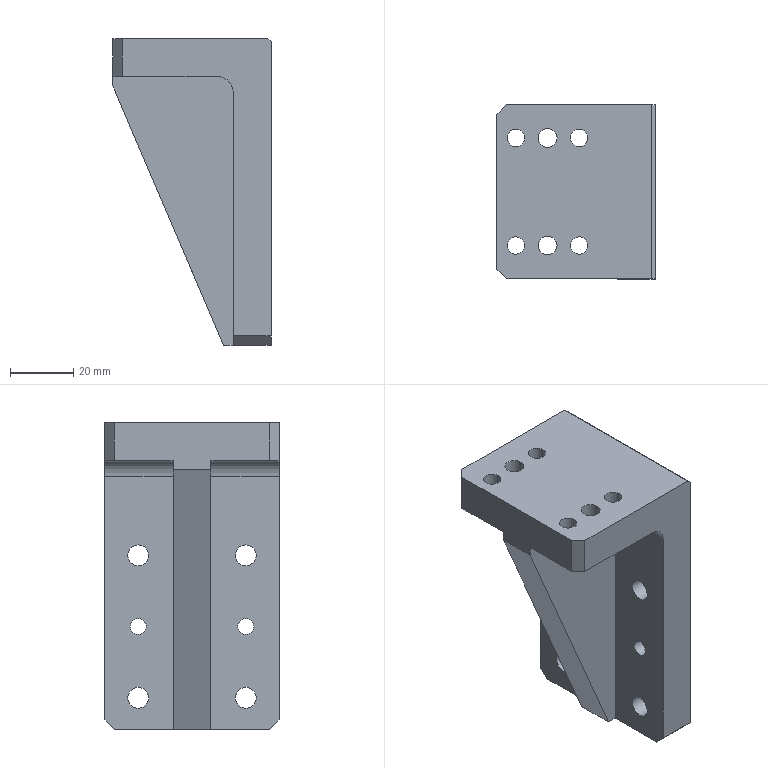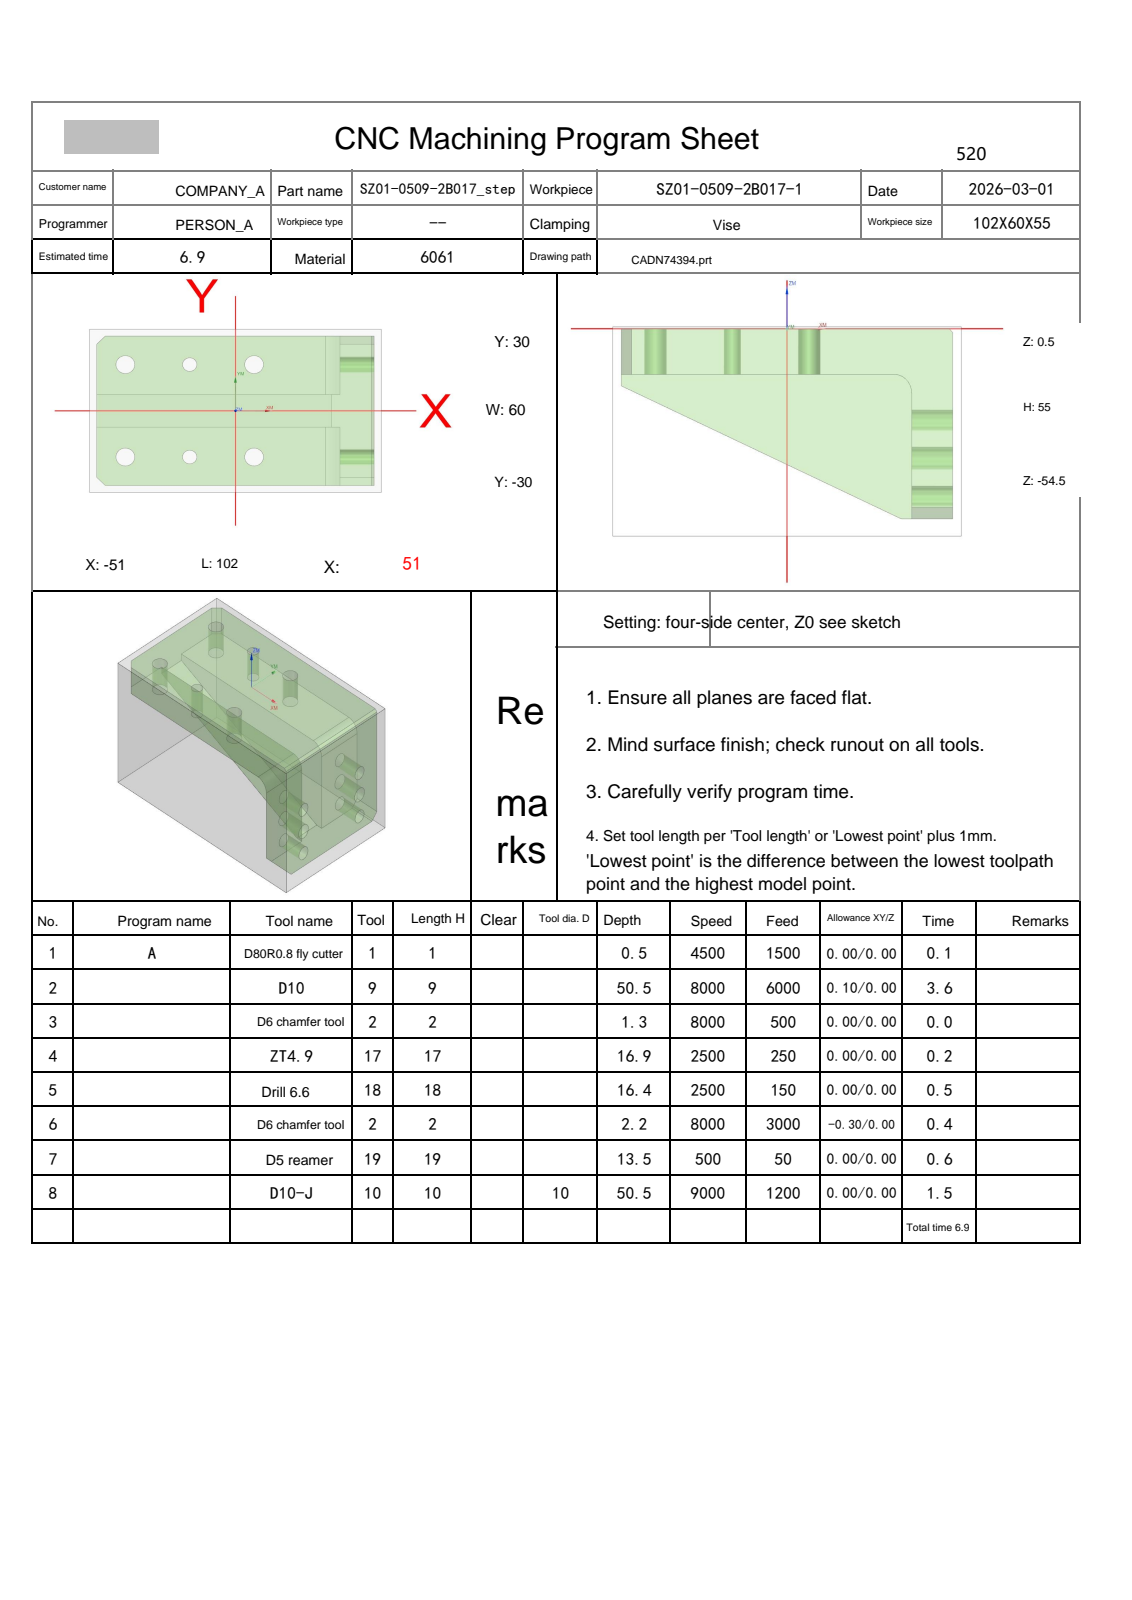NC program | NX | posted by the shop | part box 50 x 55 x 97 mm
Whole program:
%
O0001
(Machine time: 8.45 MIN)
(===Total Tool:7===)
(T1=D80R0.8 fly cutter D=80.  R=0.8  D-  H01 Z=0.    )
(T9=D10     D=10.  R=0.   D-  H09 Z=-50.  )
(T2=D6 chamfer tool   D=6.   R=0.   D-  H02 Z=-1.7  )
(T17=ZT4.9  D=4.9  DR_a=120 D-  H17 Z=-16.41)
(T18=Drill 6.6  D=6.6  DR_a=120 D-  H18 Z=-15.91)
(T19=D5 reamer   D=5.   DR_a=180 D-  H19 Z=-13.  )
(T10=D10-J  D=10.  R=0.   D10 H10 Z=-50.  )
G80 G90 G17 G49 G40
G91 G28 Z0
M01
N1 T01 M06
(D80R0.8 fly cutter  D=80. R=0.8 H=01 ce=0.00 di=0.00)
G00 G90 G54 X93.5 Y0.0 M03 S4500
G43 H01 Z50.
M08
Z2.
G01 Z0.0 F1500.
X88.5
X-88.5
X-93.5
Z2.
G00 Z50.
G91 G28 Z0.0
M05
M09
G91 G28 Z0.0
M01
N2 T09 M06
(D10  D=10. R=0. H=09 ce=0.10 di=0.00)
G00 G90 G54 X1.5 Y32.6 M03 S8000
G43 H09 Z50.
M08
Z.5
G01 X48.5 Z.388 F6000.
G02 X53.6 Y27.5 Z.369 I0.0 J-5.1
G01 Y-27.5 Z.239
G02 X48.5 Y-32.6 Z.22 I-5.1 J0.0
G01 X-45.5 Z-.003
G02 X-49.106 Y-31.106 Z-.013 I0.0 J5.1
G01 X-52.106 Y-28.106 Z-.023
G02 X-53.6 Y-24.5 Z-.032 I3.606 J3.606
G01 Y24.5 Z-.148
G02 X-52.106 Y28.106 Z-.158 I5.1 J0.0
G01 X-49.106 Y31.106 Z-.168
G02 X-45.5 Y32.6 Z-.178 I3.606 J-3.606
G01 X48.5 Z-.401
G02 X53.6 Y27.5 Z-.42 I0.0 J-5.1
G01 Y-27.5 Z-.55
G02 X48.5 Y-32.6 Z-.569 I-5.1 J0.0
G01 X-45.5 Z-.792
G02 X-49.106 Y-31.106 Z-.802 I0.0 J5.1
G01 X-52.106 Y-28.106 Z-.812
G02 X-53.6 Y-24.5 Z-.821 I3.606 J3.606
G01 Y24.5 Z-.938
G02 X-52.106 Y28.106 Z-.947 I5.1 J0.0
G01 X-49.106 Y31.106 Z-.957
G02 X-45.5 Y32.6 Z-.967 I3.606 J-3.606
G01 X48.5 Z-1.19
G02 X53.6 Y27.5 Z-1.209 I0.0 J-5.1
G01 Y-27.5 Z-1.339
G02 X48.5 Y-32.6 Z-1.358 I-5.1 J0.0
G01 X-45.5 Z-1.581
G02 X-49.106 Y-31.106 Z-1.591 I0.0 J5.1
G01 X-52.106 Y-28.106 Z-1.601
G02 X-53.6 Y-24.5 Z-1.61 I3.606 J3.606
G01 Y24.5 Z-1.727
G02 X-52.106 Y28.106 Z-1.736 I5.1 J0.0
G01 X-49.106 Y31.106 Z-1.746
G02 X-45.5 Y32.6 Z-1.756 I3.606 J-3.606
G01 X48.5 Z-1.979
G02 X53.6 Y27.5 Z-1.998 I0.0 J-5.1
G01 Y-27.5 Z-2.128
G02 X48.5 Y-32.6 Z-2.147 I-5.1 J0.0
G01 X-45.5 Z-2.37
G02 X-49.106 Y-31.106 Z-2.38 I0.0 J5.1
G01 X-52.106 Y-28.106 Z-2.39
G02 X-53.6 Y-24.5 Z-2.399 I3.606 J3.606
G01 Y24.5 Z-2.516
G02 X-52.106 Y28.106 Z-2.525 I5.1 J0.0
G01 X-49.106 Y31.106 Z-2.535
G02 X-45.5 Y32.6 Z-2.545 I3.606 J-3.606
G01 X48.5 Z-2.768
G02 X53.6 Y27.5 Z-2.787 I0.0 J-5.1
G01 Y-27.5 Z-2.917
G02 X48.5 Y-32.6 Z-2.936 I-5.1 J0.0
G01 X-45.5 Z-3.159
G02 X-49.106 Y-31.106 Z-3.169 I0.0 J5.1
G01 X-52.106 Y-28.106 Z-3.179
G02 X-53.6 Y-24.5 Z-3.188 I3.606 J3.606
G01 Y24.5 Z-3.305
G02 X-52.106 Y28.106 Z-3.314 I5.1 J0.0
G01 X-49.106 Y31.106 Z-3.324
G02 X-45.5 Y32.6 Z-3.334 I3.606 J-3.606
G01 X48.5 Z-3.557
G02 X53.6 Y27.5 Z-3.576 I0.0 J-5.1
G01 Y-27.5 Z-3.706
G02 X48.5 Y-32.6 Z-3.725 I-5.1 J0.0
G01 X-45.5 Z-3.948
G02 X-49.106 Y-31.106 Z-3.958 I0.0 J5.1
G01 X-52.106 Y-28.106 Z-3.968
G02 X-53.6 Y-24.5 Z-3.977 I3.606 J3.606
G01 Y24.5 Z-4.094
G02 X-52.106 Y28.106 Z-4.103 I5.1 J0.0
G01 X-49.106 Y31.106 Z-4.113
G02 X-45.5 Y32.6 Z-4.123 I3.606 J-3.606
G01 X48.5 Z-4.346
G02 X53.6 Y27.5 Z-4.365 I0.0 J-5.1
G01 Y-27.5 Z-4.495
G02 X48.5 Y-32.6 Z-4.514 I-5.1 J0.0
G01 X-45.5 Z-4.737
G02 X-49.106 Y-31.106 Z-4.747 I0.0 J5.1
G01 X-52.106 Y-28.106 Z-4.757
G02 X-53.6 Y-24.5 Z-4.767 I3.606 J3.606
G01 Y24.5 Z-4.883
G02 X-52.106 Y28.106 Z-4.892 I5.1 J0.0
G01 X-49.106 Y31.106 Z-4.902
G02 X-45.5 Y32.6 Z-4.912 I3.606 J-3.606
G01 X48.5 Z-5.135
G02 X53.6 Y27.5 Z-5.154 I0.0 J-5.1
G01 Y-27.5 Z-5.284
G02 X48.5 Y-32.6 Z-5.303 I-5.1 J0.0
G01 X-45.5 Z-5.527
G02 X-49.106 Y-31.106 Z-5.536 I0.0 J5.1
G01 X-52.106 Y-28.106 Z-5.546
G02 X-53.6 Y-24.5 Z-5.556 I3.606 J3.606
G01 Y24.5 Z-5.672
G02 X-52.106 Y28.106 Z-5.681 I5.1 J0.0
G01 X-49.106 Y31.106 Z-5.691
G02 X-45.5 Y32.6 Z-5.701 I3.606 J-3.606
G01 X48.5 Z-5.924
G02 X53.6 Y27.5 Z-5.943 I0.0 J-5.1
G01 Y-27.5 Z-6.074
G02 X48.5 Y-32.6 Z-6.093 I-5.1 J0.0
G01 X-45.5 Z-6.316
G02 X-49.106 Y-31.106 Z-6.325 I0.0 J5.1
G01 X-52.106 Y-28.106 Z-6.335
G02 X-53.6 Y-24.5 Z-6.345 I3.606 J3.606
G01 Y24.5 Z-6.461
G02 X-52.106 Y28.106 Z-6.47 I5.1 J0.0
G01 X-49.106 Y31.106 Z-6.481
G02 X-45.5 Y32.6 Z-6.49 I3.606 J-3.606
G01 X48.5 Z-6.713
G02 X53.6 Y27.5 Z-6.732 I0.0 J-5.1
G01 Y-27.5 Z-6.863
G02 X48.5 Y-32.6 Z-6.882 I-5.1 J0.0
G01 X-45.5 Z-7.105
G02 X-49.106 Y-31.106 Z-7.114 I0.0 J5.1
G01 X-52.106 Y-28.106 Z-7.124
G02 X-53.6 Y-24.5 Z-7.134 I3.606 J3.606
G01 Y24.5 Z-7.25
G02 X-52.106 Y28.106 Z-7.26 I5.1 J0.0
G01 X-49.106 Y31.106 Z-7.27
G02 X-45.5 Y32.6 Z-7.279 I3.606 J-3.606
G01 X48.5 Z-7.502
G02 X53.6 Y27.5 Z-7.521 I0.0 J-5.1
G01 Y-27.5 Z-7.652
G02 X48.5 Y-32.6 Z-7.671 I-5.1 J0.0
G01 X-45.5 Z-7.894
G02 X-49.106 Y-31.106 Z-7.903 I0.0 J5.1
G01 X-52.106 Y-28.106 Z-7.913
G02 X-53.6 Y-24.5 Z-7.923 I3.606 J3.606
G01 Y24.5 Z-8.039
G02 X-52.106 Y28.106 Z-8.049 I5.1 J0.0
G01 X-49.106 Y31.106 Z-8.059
G02 X-45.5 Y32.6 Z-8.068 I3.606 J-3.606
G01 X48.5 Z-8.291
G02 X53.6 Y27.5 Z-8.31 I0.0 J-5.1
G01 Y-27.5 Z-8.441
G02 X48.5 Y-32.6 Z-8.46 I-5.1 J0.0
G01 X-45.5 Z-8.683
G02 X-49.106 Y-31.106 Z-8.692 I0.0 J5.1
G01 X-52.106 Y-28.106 Z-8.702
G02 X-53.6 Y-24.5 Z-8.712 I3.606 J3.606
G01 Y24.5 Z-8.828
G02 X-52.106 Y28.106 Z-8.838 I5.1 J0.0
G01 X-49.106 Y31.106 Z-8.848
G02 X-45.5 Y32.6 Z-8.857 I3.606 J-3.606
G01 X48.5 Z-9.08
G02 X53.6 Y27.5 Z-9.099 I0.0 J-5.1
G01 Y-27.5 Z-9.23
G02 X48.5 Y-32.6 Z-9.249 I-5.1 J0.0
G01 X-45.5 Z-9.472
G02 X-49.106 Y-31.106 Z-9.481 I0.0 J5.1
G01 X-52.106 Y-28.106 Z-9.491
G02 X-53.6 Y-24.5 Z-9.501 I3.606 J3.606
G01 Y24.5 Z-9.617
G02 X-52.106 Y28.106 Z-9.627 I5.1 J0.0
G01 X-49.106 Y31.106 Z-9.637
G02 X-45.5 Y32.6 Z-9.646 I3.606 J-3.606
G01 X48.5 Z-9.869
G02 X53.6 Y27.5 Z-9.888 I0.0 J-5.1
G01 Y-27.5 Z-10.019
G02 X48.5 Y-32.6 Z-10.038 I-5.1 J0.0
G01 X-45.5 Z-10.261
G02 X-49.106 Y-31.106 Z-10.27 I0.0 J5.1
G01 X-52.106 Y-28.106 Z-10.28
G02 X-53.6 Y-24.5 Z-10.29 I3.606 J3.606
G01 Y24.5 Z-10.406
G02 X-52.106 Y28.106 Z-10.416 I5.1 J0.0
G01 X-49.106 Y31.106 Z-10.426
G02 X-45.5 Y32.6 Z-10.435 I3.606 J-3.606
G01 X48.5 Z-10.658
G02 X53.6 Y27.5 Z-10.677 I0.0 J-5.1
G01 Y-27.5 Z-10.808
G02 X48.5 Y-32.6 Z-10.827 I-5.1 J0.0
G01 X-45.5 Z-11.05
G02 X-49.106 Y-31.106 Z-11.059 I0.0 J5.1
G01 X-52.106 Y-28.106 Z-11.07
G02 X-53.6 Y-24.5 Z-11.079 I3.606 J3.606
G01 Y24.5 Z-11.195
G02 X-52.106 Y28.106 Z-11.205 I5.1 J0.0
G01 X-49.106 Y31.106 Z-11.215
G02 X-45.5 Y32.6 Z-11.224 I3.606 J-3.606
G01 X48.5 Z-11.447
G02 X53.6 Y27.5 Z-11.466 I0.0 J-5.1
G01 Y-27.5 Z-11.597
G02 X48.5 Y-32.6 Z-11.616 I-5.1 J0.0
G01 X-45.5 Z-11.839
G02 X-49.106 Y-31.106 Z-11.849 I0.0 J5.1
G01 X-52.106 Y-28.106 Z-11.859
G02 X-53.6 Y-24.5 Z-11.868 I3.606 J3.606
G01 Y24.5 Z-11.984
G02 X-52.106 Y28.106 Z-11.994 I5.1 J0.0
G01 X-49.106 Y31.106 Z-12.004
G02 X-45.5 Y32.6 Z-12.013 I3.606 J-3.606
G01 X48.5 Z-12.237
G02 X53.6 Y27.5 Z-12.256 I0.0 J-5.1
G01 Y-27.5 Z-12.386
G02 X48.5 Y-32.6 Z-12.405 I-5.1 J0.0
G01 X-45.5 Z-12.628
G02 X-49.106 Y-31.106 Z-12.638 I0.0 J5.1
G01 X-52.106 Y-28.106 Z-12.648
G02 X-53.6 Y-24.5 Z-12.657 I3.606 J3.606
G01 Y24.5 Z-12.773
G02 X-52.106 Y28.106 Z-12.783 I5.1 J0.0
G01 X-49.106 Y31.106 Z-12.793
G02 X-45.5 Y32.6 Z-12.803 I3.606 J-3.606
G01 X48.5 Z-13.026
G02 X53.6 Y27.5 Z-13.045 I0.0 J-5.1
G01 Y-27.5 Z-13.175
G02 X48.5 Y-32.6 Z-13.194 I-5.1 J0.0
G01 X-45.5 Z-13.417
G02 X-49.106 Y-31.106 Z-13.427 I0.0 J5.1
G01 X-52.106 Y-28.106 Z-13.437
G02 X-53.6 Y-24.5 Z-13.446 I3.606 J3.606
G01 Y24.5 Z-13.563
G02 X-52.106 Y28.106 Z-13.572 I5.1 J0.0
G01 X-49.106 Y31.106 Z-13.582
G02 X-45.5 Y32.6 Z-13.592 I3.606 J-3.606
G01 X48.5 Z-13.815
G02 X53.6 Y27.5 Z-13.834 I0.0 J-5.1
G01 Y-27.5 Z-13.964
G02 X48.5 Y-32.6 Z-13.983 I-5.1 J0.0
G01 X-45.5 Z-14.206
G02 X-49.106 Y-31.106 Z-14.216 I0.0 J5.1
G01 X-52.106 Y-28.106 Z-14.226
G02 X-53.6 Y-24.5 Z-14.235 I3.606 J3.606
G01 Y24.5 Z-14.352
G02 X-52.106 Y28.106 Z-14.361 I5.1 J0.0
G01 X-49.106 Y31.106 Z-14.371
G02 X-45.5 Y32.6 Z-14.381 I3.606 J-3.606
G01 X48.5 Z-14.604
G02 X53.6 Y27.5 Z-14.623 I0.0 J-5.1
G01 Y-27.5 Z-14.753
G02 X48.5 Y-32.6 Z-14.772 I-5.1 J0.0
G01 X-45.5 Z-14.995
G02 X-49.106 Y-31.106 Z-15.005 I0.0 J5.1
G01 X-52.106 Y-28.106 Z-15.015
G02 X-53.6 Y-24.5 Z-15.024 I3.606 J3.606
G01 Y24.5 Z-15.141
G02 X-52.106 Y28.106 Z-15.15 I5.1 J0.0
G01 X-49.106 Y31.106 Z-15.16
G02 X-45.5 Y32.6 Z-15.17 I3.606 J-3.606
G01 X48.5 Z-15.393
G02 X53.6 Y27.5 Z-15.412 I0.0 J-5.1
G01 Y-27.5 Z-15.542
G02 X48.5 Y-32.6 Z-15.561 I-5.1 J0.0
G01 X-45.5 Z-15.784
G02 X-49.106 Y-31.106 Z-15.794 I0.0 J5.1
G01 X-52.106 Y-28.106 Z-15.804
G02 X-53.6 Y-24.5 Z-15.813 I3.606 J3.606
G01 Y24.5 Z-15.93
G02 X-52.106 Y28.106 Z-15.939 I5.1 J0.0
G01 X-49.106 Y31.106 Z-15.949
G02 X-45.5 Y32.6 Z-15.959 I3.606 J-3.606
G01 X48.5 Z-16.182
G02 X53.6 Y27.5 Z-16.201 I0.0 J-5.1
G01 Y-27.5 Z-16.331
G02 X48.5 Y-32.6 Z-16.35 I-5.1 J0.0
G01 X-45.5 Z-16.573
G02 X-49.106 Y-31.106 Z-16.583 I0.0 J5.1
G01 X-52.106 Y-28.106 Z-16.593
G02 X-53.6 Y-24.5 Z-16.602 I3.606 J3.606
G01 Y24.5 Z-16.719
G02 X-52.106 Y28.106 Z-16.728 I5.1 J0.0
G01 X-49.106 Y31.106 Z-16.738
G02 X-45.5 Y32.6 Z-16.748 I3.606 J-3.606
G01 X48.5 Z-16.971
G02 X53.6 Y27.5 Z-16.99 I0.0 J-5.1
G01 Y-27.5 Z-17.12
G02 X48.5 Y-32.6 Z-17.139 I-5.1 J0.0
G01 X-45.5 Z-17.362
G02 X-49.106 Y-31.106 Z-17.372 I0.0 J5.1
G01 X-52.106 Y-28.106 Z-17.382
G02 X-53.6 Y-24.5 Z-17.392 I3.606 J3.606
G01 Y24.5 Z-17.508
G02 X-52.106 Y28.106 Z-17.517 I5.1 J0.0
G01 X-49.106 Y31.106 Z-17.527
G02 X-45.5 Y32.6 Z-17.537 I3.606 J-3.606
G01 X48.5 Z-17.76
G02 X53.6 Y27.5 Z-17.779 I0.0 J-5.1
G01 Y-27.5 Z-17.909
G02 X48.5 Y-32.6 Z-17.928 I-5.1 J0.0
G01 X-45.5 Z-18.152
G02 X-49.106 Y-31.106 Z-18.161 I0.0 J5.1
G01 X-52.106 Y-28.106 Z-18.171
G02 X-53.6 Y-24.5 Z-18.181 I3.606 J3.606
G01 Y24.5 Z-18.297
G02 X-52.106 Y28.106 Z-18.306 I5.1 J0.0
G01 X-49.106 Y31.106 Z-18.316
G02 X-45.5 Y32.6 Z-18.326 I3.606 J-3.606
G01 X48.5 Z-18.549
G02 X53.6 Y27.5 Z-18.568 I0.0 J-5.1
G01 Y-27.5 Z-18.699
G02 X48.5 Y-32.6 Z-18.718 I-5.1 J0.0
G01 X-45.5 Z-18.941
G02 X-49.106 Y-31.106 Z-18.95 I0.0 J5.1
G01 X-52.106 Y-28.106 Z-18.96
G02 X-53.6 Y-24.5 Z-18.97 I3.606 J3.606
G01 Y24.5 Z-19.086
G02 X-52.106 Y28.106 Z-19.095 I5.1 J0.0
G01 X-49.106 Y31.106 Z-19.106
G02 X-45.5 Y32.6 Z-19.115 I3.606 J-3.606
G01 X48.5 Z-19.338
G02 X53.6 Y27.5 Z-19.357 I0.0 J-5.1
G01 Y-27.5 Z-19.488
G02 X48.5 Y-32.6 Z-19.507 I-5.1 J0.0
G01 X-45.5 Z-19.73
G02 X-49.106 Y-31.106 Z-19.739 I0.0 J5.1
G01 X-52.106 Y-28.106 Z-19.749
G02 X-53.6 Y-24.5 Z-19.759 I3.606 J3.606
G01 Y24.5 Z-19.875
G02 X-52.106 Y28.106 Z-19.885 I5.1 J0.0
G01 X-49.106 Y31.106 Z-19.895
G02 X-45.5 Y32.6 Z-19.904 I3.606 J-3.606
G01 X48.5 Z-20.127
G02 X53.6 Y27.5 Z-20.146 I0.0 J-5.1
G01 Y-27.5 Z-20.277
G02 X48.5 Y-32.6 Z-20.296 I-5.1 J0.0
G01 X-45.5 Z-20.519
G02 X-49.106 Y-31.106 Z-20.528 I0.0 J5.1
G01 X-52.106 Y-28.106 Z-20.538
G02 X-53.6 Y-24.5 Z-20.548 I3.606 J3.606
G01 Y24.5 Z-20.664
G02 X-52.106 Y28.106 Z-20.674 I5.1 J0.0
G01 X-49.106 Y31.106 Z-20.684
G02 X-45.5 Y32.6 Z-20.693 I3.606 J-3.606
G01 X48.5 Z-20.916
G02 X53.6 Y27.5 Z-20.935 I0.0 J-5.1
G01 Y-27.5 Z-21.066
G02 X48.5 Y-32.6 Z-21.085 I-5.1 J0.0
G01 X-45.5 Z-21.308
G02 X-49.106 Y-31.106 Z-21.317 I0.0 J5.1
G01 X-52.106 Y-28.106 Z-21.327
G02 X-53.6 Y-24.5 Z-21.337 I3.606 J3.606
G01 Y24.5 Z-21.453
G02 X-52.106 Y28.106 Z-21.463 I5.1 J0.0
G01 X-49.106 Y31.106 Z-21.473
G02 X-45.5 Y32.6 Z-21.482 I3.606 J-3.606
G01 X48.5 Z-21.705
G02 X53.6 Y27.5 Z-21.724 I0.0 J-5.1
G01 Y-27.5 Z-21.855
G02 X48.5 Y-32.6 Z-21.874 I-5.1 J0.0
G01 X-45.5 Z-22.097
G02 X-49.106 Y-31.106 Z-22.106 I0.0 J5.1
G01 X-52.106 Y-28.106 Z-22.116
G02 X-53.6 Y-24.5 Z-22.126 I3.606 J3.606
G01 Y24.5 Z-22.242
G02 X-52.106 Y28.106 Z-22.252 I5.1 J0.0
G01 X-49.106 Y31.106 Z-22.262
G02 X-45.5 Y32.6 Z-22.271 I3.606 J-3.606
G01 X48.5 Z-22.494
G02 X53.6 Y27.5 Z-22.513 I0.0 J-5.1
G01 Y-27.5 Z-22.644
G02 X48.5 Y-32.6 Z-22.663 I-5.1 J0.0
G01 X-45.5 Z-22.886
G02 X-49.106 Y-31.106 Z-22.895 I0.0 J5.1
G01 X-52.106 Y-28.106 Z-22.905
G02 X-53.6 Y-24.5 Z-22.915 I3.606 J3.606
G01 Y24.5 Z-23.031
G02 X-52.106 Y28.106 Z-23.041 I5.1 J0.0
G01 X-49.106 Y31.106 Z-23.051
G02 X-45.5 Y32.6 Z-23.06 I3.606 J-3.606
G01 X48.5 Z-23.283
G02 X53.6 Y27.5 Z-23.302 I0.0 J-5.1
G01 Y-27.5 Z-23.433
G02 X48.5 Y-32.6 Z-23.452 I-5.1 J0.0
G01 X-45.5 Z-23.675
G02 X-49.106 Y-31.106 Z-23.684 I0.0 J5.1
G01 X-52.106 Y-28.106 Z-23.695
G02 X-53.6 Y-24.5 Z-23.704 I3.606 J3.606
G01 Y24.5 Z-23.82
G02 X-52.106 Y28.106 Z-23.83 I5.1 J0.0
G01 X-49.106 Y31.106 Z-23.84
G02 X-45.5 Y32.6 Z-23.849 I3.606 J-3.606
G01 X48.5 Z-24.072
G02 X53.6 Y27.5 Z-24.091 I0.0 J-5.1
G01 Y-27.5 Z-24.222
G02 X48.5 Y-32.6 Z-24.241 I-5.1 J0.0
G01 X-45.5 Z-24.464
G02 X-49.106 Y-31.106 Z-24.474 I0.0 J5.1
G01 X-52.106 Y-28.106 Z-24.484
G02 X-53.6 Y-24.5 Z-24.493 I3.606 J3.606
G01 Y24.5 Z-24.609
G02 X-52.106 Y28.106 Z-24.619 I5.1 J0.0
G01 X-49.106 Y31.106 Z-24.629
G02 X-45.5 Y32.6 Z-24.638 I3.606 J-3.606
G01 X48.5 Z-24.862
G02 X53.6 Y27.5 Z-24.881 I0.0 J-5.1
G01 Y-27.5 Z-25.011
G02 X48.5 Y-32.6 Z-25.03 I-5.1 J0.0
G01 X-45.5 Z-25.253
G02 X-49.106 Y-31.106 Z-25.263 I0.0 J5.1
G01 X-52.106 Y-28.106 Z-25.273
G02 X-53.6 Y-24.5 Z-25.282 I3.606 J3.606
G01 Y24.5 Z-25.398
G02 X-52.106 Y28.106 Z-25.408 I5.1 J0.0
G01 X-49.106 Y31.106 Z-25.418
G02 X-45.5 Y32.6 Z-25.428 I3.606 J-3.606
G01 X48.5 Z-25.651
G02 X53.6 Y27.5 Z-25.67 I0.0 J-5.1
G01 Y-27.5 Z-25.8
G02 X48.5 Y-32.6 Z-25.819 I-5.1 J0.0
G01 X-45.5 Z-26.042
G02 X-49.106 Y-31.106 Z-26.052 I0.0 J5.1
G01 X-52.106 Y-28.106 Z-26.062
G02 X-53.6 Y-24.5 Z-26.071 I3.606 J3.606
G01 Y24.5 Z-26.188
G02 X-52.106 Y28.106 Z-26.197 I5.1 J0.0
G01 X-49.106 Y31.106 Z-26.207
G02 X-45.5 Y32.6 Z-26.217 I3.606 J-3.606
G01 X48.5 Z-26.44
G02 X53.6 Y27.5 Z-26.459 I0.0 J-5.1
G01 Y-27.5 Z-26.589
G02 X48.5 Y-32.6 Z-26.608 I-5.1 J0.0
G01 X-45.5 Z-26.831
G02 X-49.106 Y-31.106 Z-26.841 I0.0 J5.1
G01 X-52.106 Y-28.106 Z-26.851
G02 X-53.6 Y-24.5 Z-26.86 I3.606 J3.606
G01 Y24.5 Z-26.977
G02 X-52.106 Y28.106 Z-26.986 I5.1 J0.0
G01 X-49.106 Y31.106 Z-26.996
G02 X-45.5 Y32.6 Z-27.006 I3.606 J-3.606
G01 X48.5 Z-27.229
G02 X53.6 Y27.5 Z-27.248 I0.0 J-5.1
G01 Y-27.5 Z-27.378
G02 X48.5 Y-32.6 Z-27.397 I-5.1 J0.0
G01 X-45.5 Z-27.62
G02 X-49.106 Y-31.106 Z-27.63 I0.0 J5.1
G01 X-52.106 Y-28.106 Z-27.64
G02 X-53.6 Y-24.5 Z-27.649 I3.606 J3.606
G01 Y24.5 Z-27.766
G02 X-52.106 Y28.106 Z-27.775 I5.1 J0.0
G01 X-49.106 Y31.106 Z-27.785
G02 X-45.5 Y32.6 Z-27.795 I3.606 J-3.606
G01 X48.5 Z-28.018
G02 X53.6 Y27.5 Z-28.037 I0.0 J-5.1
G01 Y-27.5 Z-28.167
G02 X48.5 Y-32.6 Z-28.186 I-5.1 J0.0
G01 X-45.5 Z-28.409
G02 X-49.106 Y-31.106 Z-28.419 I0.0 J5.1
G01 X-52.106 Y-28.106 Z-28.429
G02 X-53.6 Y-24.5 Z-28.438 I3.606 J3.606
G01 Y24.5 Z-28.555
G02 X-52.106 Y28.106 Z-28.564 I5.1 J0.0
G01 X-49.106 Y31.106 Z-28.574
G02 X-45.5 Y32.6 Z-28.584 I3.606 J-3.606
G01 X48.5 Z-28.807
G02 X53.6 Y27.5 Z-28.826 I0.0 J-5.1
G01 Y-27.5 Z-28.956
G02 X48.5 Y-32.6 Z-28.975 I-5.1 J0.0
G01 X-45.5 Z-29.198
G02 X-49.106 Y-31.106 Z-29.208 I0.0 J5.1
G01 X-52.106 Y-28.106 Z-29.218
G02 X-53.6 Y-24.5 Z-29.227 I3.606 J3.606
G01 Y24.5 Z-29.344
G02 X-52.106 Y28.106 Z-29.353 I5.1 J0.0
G01 X-49.106 Y31.106 Z-29.363
G02 X-45.5 Y32.6 Z-29.373 I3.606 J-3.606
G01 X48.5 Z-29.596
G02 X53.6 Y27.5 Z-29.615 I0.0 J-5.1
G01 Y-27.5 Z-29.745
G02 X48.5 Y-32.6 Z-29.764 I-5.1 J0.0
G01 X-45.5 Z-29.987
G02 X-49.106 Y-31.106 Z-29.997 I0.0 J5.1
G01 X-52.106 Y-28.106 Z-30.007
G02 X-53.6 Y-24.5 Z-30.017 I3.606 J3.606
G01 Y24.5 Z-30.133
G02 X-52.106 Y28.106 Z-30.142 I5.1 J0.0
G01 X-49.106 Y31.106 Z-30.152
G02 X-45.5 Y32.6 Z-30.162 I3.606 J-3.606
G01 X48.5 Z-30.385
G02 X53.6 Y27.5 Z-30.404 I0.0 J-5.1
G01 Y-27.5 Z-30.534
G02 X48.5 Y-32.6 Z-30.553 I-5.1 J0.0
G01 X-45.5 Z-30.777
G02 X-49.106 Y-31.106 Z-30.786 I0.0 J5.1
G01 X-52.106 Y-28.106 Z-30.796
G02 X-53.6 Y-24.5 Z-30.806 I3.606 J3.606
G01 Y24.5 Z-30.922
G02 X-52.106 Y28.106 Z-30.931 I5.1 J0.0
G01 X-49.106 Y31.106 Z-30.941
G02 X-45.5 Y32.6 Z-30.951 I3.606 J-3.606
G01 X48.5 Z-31.174
G02 X53.6 Y27.5 Z-31.193 I0.0 J-5.1
G01 Y-27.5 Z-31.324
G02 X48.5 Y-32.6 Z-31.343 I-5.1 J0.0
G01 X-45.5 Z-31.566
G02 X-49.106 Y-31.106 Z-31.575 I0.0 J5.1
G01 X-52.106 Y-28.106 Z-31.585
G02 X-53.6 Y-24.5 Z-31.595 I3.606 J3.606
G01 Y24.5 Z-31.711
G02 X-52.106 Y28.106 Z-31.72 I5.1 J0.0
G01 X-49.106 Y31.106 Z-31.731
G02 X-45.5 Y32.6 Z-31.74 I3.606 J-3.606
G01 X48.5 Z-31.963
G02 X53.6 Y27.5 Z-31.982 I0.0 J-5.1
G01 Y-27.5 Z-32.113
G02 X48.5 Y-32.6 Z-32.132 I-5.1 J0.0
G01 X-45.5 Z-32.355
G02 X-49.106 Y-31.106 Z-32.364 I0.0 J5.1
G01 X-52.106 Y-28.106 Z-32.374
G02 X-53.6 Y-24.5 Z-32.384 I3.606 J3.606
G01 Y24.5 Z-32.5
G02 X-52.106 Y28.106 Z-32.51 I5.1 J0.0
G01 X-49.106 Y31.106 Z-32.52
G02 X-45.5 Y32.6 Z-32.529 I3.606 J-3.606
G01 X48.5 Z-32.752
G02 X53.6 Y27.5 Z-32.771 I0.0 J-5.1
G01 Y-27.5 Z-32.902
G02 X48.5 Y-32.6 Z-32.921 I-5.1 J0.0
G01 X-45.5 Z-33.144
G02 X-49.106 Y-31.106 Z-33.153 I0.0 J5.1
G01 X-52.106 Y-28.106 Z-33.163
G02 X-53.6 Y-24.5 Z-33.173 I3.606 J3.606
G01 Y24.5 Z-33.289
G02 X-52.106 Y28.106 Z-33.299 I5.1 J0.0
G01 X-49.106 Y31.106 Z-33.309
G02 X-45.5 Y32.6 Z-33.318 I3.606 J-3.606
G01 X48.5 Z-33.541
G02 X53.6 Y27.5 Z-33.56 I0.0 J-5.1
G01 Y-27.5 Z-33.691
G02 X48.5 Y-32.6 Z-33.71 I-5.1 J0.0
G01 X-45.5 Z-33.933
G02 X-49.106 Y-31.106 Z-33.942 I0.0 J5.1
G01 X-52.106 Y-28.106 Z-33.952
G02 X-53.6 Y-24.5 Z-33.962 I3.606 J3.606
G01 Y24.5 Z-34.078
G02 X-52.106 Y28.106 Z-34.088 I5.1 J0.0
G01 X-49.106 Y31.106 Z-34.098
G02 X-45.5 Y32.6 Z-34.107 I3.606 J-3.606
G01 X48.5 Z-34.33
G02 X53.6 Y27.5 Z-34.349 I0.0 J-5.1
G01 Y-27.5 Z-34.48
G02 X48.5 Y-32.6 Z-34.499 I-5.1 J0.0
G01 X-45.5 Z-34.722
G02 X-49.106 Y-31.106 Z-34.731 I0.0 J5.1
G01 X-52.106 Y-28.106 Z-34.741
G02 X-53.6 Y-24.5 Z-34.751 I3.606 J3.606
G01 Y24.5 Z-34.867
G02 X-52.106 Y28.106 Z-34.877 I5.1 J0.0
G01 X-49.106 Y31.106 Z-34.887
G02 X-45.5 Y32.6 Z-34.896 I3.606 J-3.606
G01 X48.5 Z-35.119
G02 X53.6 Y27.5 Z-35.138 I0.0 J-5.1
G01 Y-27.5 Z-35.269
G02 X48.5 Y-32.6 Z-35.288 I-5.1 J0.0
G01 X-45.5 Z-35.511
G02 X-49.106 Y-31.106 Z-35.52 I0.0 J5.1
G01 X-52.106 Y-28.106 Z-35.53
G02 X-53.6 Y-24.5 Z-35.54 I3.606 J3.606
G01 Y24.5 Z-35.656
G02 X-52.106 Y28.106 Z-35.666 I5.1 J0.0
G01 X-49.106 Y31.106 Z-35.676
G02 X-45.5 Y32.6 Z-35.685 I3.606 J-3.606
G01 X48.5 Z-35.908
G02 X53.6 Y27.5 Z-35.927 I0.0 J-5.1
G01 Y-27.5 Z-36.058
G02 X48.5 Y-32.6 Z-36.077 I-5.1 J0.0
G01 X-45.5 Z-36.3
G02 X-49.106 Y-31.106 Z-36.309 I0.0 J5.1
G01 X-52.106 Y-28.106 Z-36.32
G02 X-53.6 Y-24.5 Z-36.329 I3.606 J3.606
G01 Y24.5 Z-36.445
G02 X-52.106 Y28.106 Z-36.455 I5.1 J0.0
G01 X-49.106 Y31.106 Z-36.465
G02 X-45.5 Y32.6 Z-36.474 I3.606 J-3.606
G01 X48.5 Z-36.697
G02 X53.6 Y27.5 Z-36.716 I0.0 J-5.1
G01 Y-27.5 Z-36.847
G02 X48.5 Y-32.6 Z-36.866 I-5.1 J0.0
G01 X-45.5 Z-37.089
G02 X-49.106 Y-31.106 Z-37.099 I0.0 J5.1
G01 X-52.106 Y-28.106 Z-37.109
G02 X-53.6 Y-24.5 Z-37.118 I3.606 J3.606
G01 Y24.5 Z-37.234
G02 X-52.106 Y28.106 Z-37.244 I5.1 J0.0
G01 X-49.106 Y31.106 Z-37.254
G02 X-45.5 Y32.6 Z-37.263 I3.606 J-3.606
G01 X48.5 Z-37.487
G02 X53.6 Y27.5 Z-37.506 I0.0 J-5.1
G01 Y-27.5 Z-37.636
G02 X48.5 Y-32.6 Z-37.655 I-5.1 J0.0
G01 X-45.5 Z-37.878
G02 X-49.106 Y-31.106 Z-37.888 I0.0 J5.1
G01 X-52.106 Y-28.106 Z-37.898
G02 X-53.6 Y-24.5 Z-37.907 I3.606 J3.606
G01 Y24.5 Z-38.023
G02 X-52.106 Y28.106 Z-38.033 I5.1 J0.0
G01 X-49.106 Y31.106 Z-38.043
G02 X-45.5 Y32.6 Z-38.053 I3.606 J-3.606
G01 X48.5 Z-38.276
G02 X53.6 Y27.5 Z-38.295 I0.0 J-5.1
G01 Y-27.5 Z-38.425
G02 X48.5 Y-32.6 Z-38.444 I-5.1 J0.0
G01 X-45.5 Z-38.667
G02 X-49.106 Y-31.106 Z-38.677 I0.0 J5.1
G01 X-52.106 Y-28.106 Z-38.687
G02 X-53.6 Y-24.5 Z-38.696 I3.606 J3.606
G01 Y24.5 Z-38.813
G02 X-52.106 Y28.106 Z-38.822 I5.1 J0.0
G01 X-49.106 Y31.106 Z-38.832
G02 X-45.5 Y32.6 Z-38.842 I3.606 J-3.606
G01 X48.5 Z-39.065
G02 X53.6 Y27.5 Z-39.084 I0.0 J-5.1
G01 Y-27.5 Z-39.214
G02 X48.5 Y-32.6 Z-39.233 I-5.1 J0.0
G01 X-45.5 Z-39.456
G02 X-49.106 Y-31.106 Z-39.466 I0.0 J5.1
G01 X-52.106 Y-28.106 Z-39.476
G02 X-53.6 Y-24.5 Z-39.485 I3.606 J3.606
G01 Y24.5 Z-39.602
G02 X-52.106 Y28.106 Z-39.611 I5.1 J0.0
G01 X-49.106 Y31.106 Z-39.621
G02 X-45.5 Y32.6 Z-39.631 I3.606 J-3.606
G01 X48.5 Z-39.854
G02 X53.6 Y27.5 Z-39.873 I0.0 J-5.1
G01 Y-27.5 Z-40.003
G02 X48.5 Y-32.6 Z-40.022 I-5.1 J0.0
G01 X-45.5 Z-40.245
G02 X-49.106 Y-31.106 Z-40.255 I0.0 J5.1
G01 X-52.106 Y-28.106 Z-40.265
G02 X-53.6 Y-24.5 Z-40.274 I3.606 J3.606
G01 Y24.5 Z-40.391
G02 X-52.106 Y28.106 Z-40.4 I5.1 J0.0
G01 X-49.106 Y31.106 Z-40.41
G02 X-45.5 Y32.6 Z-40.42 I3.606 J-3.606
G01 X48.5 Z-40.643
G02 X53.6 Y27.5 Z-40.662 I0.0 J-5.1
G01 Y-27.5 Z-40.792
G02 X48.5 Y-32.6 Z-40.811 I-5.1 J0.0
G01 X-45.5 Z-41.034
G02 X-49.106 Y-31.106 Z-41.044 I0.0 J5.1
G01 X-52.106 Y-28.106 Z-41.054
G02 X-53.6 Y-24.5 Z-41.063 I3.606 J3.606
G01 Y24.5 Z-41.18
G02 X-52.106 Y28.106 Z-41.189 I5.1 J0.0
G01 X-49.106 Y31.106 Z-41.199
G02 X-45.5 Y32.6 Z-41.209 I3.606 J-3.606
G01 X48.5 Z-41.432
G02 X53.6 Y27.5 Z-41.451 I0.0 J-5.1
G01 Y-27.5 Z-41.581
G02 X48.5 Y-32.6 Z-41.6 I-5.1 J0.0
G01 X-45.5 Z-41.823
G02 X-49.106 Y-31.106 Z-41.833 I0.0 J5.1
G01 X-52.106 Y-28.106 Z-41.843
G02 X-53.6 Y-24.5 Z-41.852 I3.606 J3.606
G01 Y24.5 Z-41.969
G02 X-52.106 Y28.106 Z-41.978 I5.1 J0.0
G01 X-49.106 Y31.106 Z-41.988
G02 X-45.5 Y32.6 Z-41.998 I3.606 J-3.606
G01 X48.5 Z-42.221
G02 X53.6 Y27.5 Z-42.24 I0.0 J-5.1
G01 Y-27.5 Z-42.37
G02 X48.5 Y-32.6 Z-42.389 I-5.1 J0.0
G01 X-45.5 Z-42.612
G02 X-49.106 Y-31.106 Z-42.622 I0.0 J5.1
G01 X-52.106 Y-28.106 Z-42.632
G02 X-53.6 Y-24.5 Z-42.642 I3.606 J3.606
G01 Y24.5 Z-42.758
G02 X-52.106 Y28.106 Z-42.767 I5.1 J0.0
G01 X-49.106 Y31.106 Z-42.777
G02 X-45.5 Y32.6 Z-42.787 I3.606 J-3.606
G01 X48.5 Z-43.01
G02 X53.6 Y27.5 Z-43.029 I0.0 J-5.1
G01 Y-27.5 Z-43.159
G02 X48.5 Y-32.6 Z-43.178 I-5.1 J0.0
G01 X-45.5 Z-43.402
G02 X-49.106 Y-31.106 Z-43.411 I0.0 J5.1
G01 X-52.106 Y-28.106 Z-43.421
G02 X-53.6 Y-24.5 Z-43.431 I3.606 J3.606
G01 Y24.5 Z-43.547
G02 X-52.106 Y28.106 Z-43.556 I5.1 J0.0
G01 X-49.106 Y31.106 Z-43.566
G02 X-45.5 Y32.6 Z-43.576 I3.606 J-3.606
G01 X48.5 Z-43.799
G02 X53.6 Y27.5 Z-43.818 I0.0 J-5.1
G01 Y-27.5 Z-43.949
G02 X48.5 Y-32.6 Z-43.968 I-5.1 J0.0
G01 X-45.5 Z-44.191
G02 X-49.106 Y-31.106 Z-44.2 I0.0 J5.1
G01 X-52.106 Y-28.106 Z-44.21
G02 X-53.6 Y-24.5 Z-44.22 I3.606 J3.606
G01 Y24.5 Z-44.336
G02 X-52.106 Y28.106 Z-44.345 I5.1 J0.0
G01 X-49.106 Y31.106 Z-44.356
G02 X-45.5 Y32.6 Z-44.365 I3.606 J-3.606
G01 X48.5 Z-44.588
G02 X53.6 Y27.5 Z-44.607 I0.0 J-5.1
G01 Y-27.5 Z-44.738
G02 X48.5 Y-32.6 Z-44.757 I-5.1 J0.0
G01 X-45.5 Z-44.98
G02 X-49.106 Y-31.106 Z-44.989 I0.0 J5.1
G01 X-52.106 Y-28.106 Z-44.999
G02 X-53.6 Y-24.5 Z-45.009 I3.606 J3.606
G01 Y24.5 Z-45.125
G02 X-52.106 Y28.106 Z-45.135 I5.1 J0.0
G01 X-49.106 Y31.106 Z-45.145
G02 X-45.5 Y32.6 Z-45.154 I3.606 J-3.606
G01 X48.5 Z-45.377
G02 X53.6 Y27.5 Z-45.396 I0.0 J-5.1
G01 Y-27.5 Z-45.527
G02 X48.5 Y-32.6 Z-45.546 I-5.1 J0.0
G01 X-45.5 Z-45.769
G02 X-49.106 Y-31.106 Z-45.778 I0.0 J5.1
G01 X-52.106 Y-28.106 Z-45.788
G02 X-53.6 Y-24.5 Z-45.798 I3.606 J3.606
G01 Y24.5 Z-45.914
G02 X-52.106 Y28.106 Z-45.924 I5.1 J0.0
G01 X-49.106 Y31.106 Z-45.934
G02 X-45.5 Y32.6 Z-45.943 I3.606 J-3.606
G01 X48.5 Z-46.166
G02 X53.6 Y27.5 Z-46.185 I0.0 J-5.1
G01 Y-27.5 Z-46.316
G02 X48.5 Y-32.6 Z-46.335 I-5.1 J0.0
G01 X-45.5 Z-46.558
G02 X-49.106 Y-31.106 Z-46.567 I0.0 J5.1
G01 X-52.106 Y-28.106 Z-46.577
G02 X-53.6 Y-24.5 Z-46.587 I3.606 J3.606
G01 Y24.5 Z-46.703
G02 X-52.106 Y28.106 Z-46.713 I5.1 J0.0
G01 X-49.106 Y31.106 Z-46.723
G02 X-45.5 Y32.6 Z-46.732 I3.606 J-3.606
G01 X48.5 Z-46.955
G02 X53.6 Y27.5 Z-46.974 I0.0 J-5.1
G01 Y-27.5 Z-47.105
G02 X48.5 Y-32.6 Z-47.124 I-5.1 J0.0
G01 X-45.5 Z-47.347
G02 X-49.106 Y-31.106 Z-47.356 I0.0 J5.1
G01 X-52.106 Y-28.106 Z-47.366
G02 X-53.6 Y-24.5 Z-47.376 I3.606 J3.606
G01 Y24.5 Z-47.492
G02 X-52.106 Y28.106 Z-47.502 I5.1 J0.0
G01 X-49.106 Y31.106 Z-47.512
G02 X-45.5 Y32.6 Z-47.521 I3.606 J-3.606
G01 X48.5 Z-47.744
G02 X53.6 Y27.5 Z-47.763 I0.0 J-5.1
G01 Y-27.5 Z-47.894
G02 X48.5 Y-32.6 Z-47.913 I-5.1 J0.0
G01 X-45.5 Z-48.136
G02 X-49.106 Y-31.106 Z-48.145 I0.0 J5.1
G01 X-52.106 Y-28.106 Z-48.155
G02 X-53.6 Y-24.5 Z-48.165 I3.606 J3.606
G01 Y24.5 Z-48.281
G02 X-52.106 Y28.106 Z-48.291 I5.1 J0.0
G01 X-49.106 Y31.106 Z-48.301
G02 X-45.5 Y32.6 Z-48.31 I3.606 J-3.606
G01 X48.5 Z-48.533
G02 X53.6 Y27.5 Z-48.552 I0.0 J-5.1
G01 Y-27.5 Z-48.683
G02 X48.5 Y-32.6 Z-48.702 I-5.1 J0.0
G01 X-45.5 Z-48.925
G02 X-49.106 Y-31.106 Z-48.934 I0.0 J5.1
G01 X-52.106 Y-28.106 Z-48.945
G02 X-53.6 Y-24.5 Z-48.954 I3.606 J3.606
G01 Y24.5 Z-49.07
G02 X-52.106 Y28.106 Z-49.08 I5.1 J0.0
G01 X-49.106 Y31.106 Z-49.09
G02 X-45.5 Y32.6 Z-49.099 I3.606 J-3.606
G01 X48.5 Z-49.322
G02 X53.6 Y27.5 Z-49.341 I0.0 J-5.1
G01 Y-27.5 Z-49.472
G02 X48.5 Y-32.6 Z-49.491 I-5.1 J0.0
G01 X-45.5 Z-49.714
G02 X-49.106 Y-31.106 Z-49.724 I0.0 J5.1
G01 X-52.106 Y-28.106 Z-49.734
G02 X-53.6 Y-24.5 Z-49.743 I3.606 J3.606
G01 Y24.5 Z-49.859
G02 X-52.106 Y28.106 Z-49.869 I5.1 J0.0
G01 X-49.106 Y31.106 Z-49.879
G02 X-45.5 Y32.6 Z-49.888 I3.606 J-3.606
G01 X1.5 Z-50.
X48.5
G02 X53.6 Y27.5 I0.0 J-5.1
G01 Y-27.5
G02 X48.5 Y-32.6 I-5.1 J0.0
G01 X-45.5
G02 X-49.106 Y-31.106 I0.0 J5.1
G01 X-52.106 Y-28.106
G02 X-53.6 Y-24.5 I3.606 J3.606
G01 Y24.5
G02 X-52.106 Y28.106 I5.1 J0.0
G01 X-49.106 Y31.106
G02 X-45.5 Y32.6 I3.606 J-3.606
G01 X1.5
X2.
Z-49.
G00 Z50.
G91 G28 Z0.0
M05
M09
G91 G28 Z0.0
M01
N3 T02 M06
(D6 chamfer tool  D=6. R=0. H=02 ce=0.00 di=0.00)
G00 G90 G54 X6.5 Y-17. M03 S8000
G43 H02 Z50.
M08
G98 G81 X6.5 Y-17. Z-.8 R1. F500.
X-16.
X-38.5
Y17.
X-16.
X6.5
G80
G00 Z50.
G91 G28 Z0.0
M05
M09
G91 G28 Z0.0
M01
N4 T17 M06
(ZT4.9 D=4.9 DR_a=120 H=17)
G00 G90 G54 X-16. Y-17. M03 S2500
G43 H17 Z50.
M08
G98 G83 X-16. Y-17. Z-16.415 R1. F250. Q2.
Y17.
G80
G00 Z50.
G91 G28 Z0.0
M05
M09
G91 G28 Z0.0
M01
N5 T18 M06
(Drill 6.6 D=6.6 DR_a=120 H=18)
G00 G90 G54 X6.5 Y-17. M03 S2500
G43 H18 Z50.
M08
G98 G83 X6.5 Y-17. Z-15.905 R1. F150. Q3.
Y17.
X-38.5
Y-17.
G80
G00 Z50.
G91 G28 Z0.0
M05
M09
G91 G28 Z0.0
M01
N6 T02 M06
(D6 chamfer tool  D=6. R=0. H=02 ce=0.00 di=0.00)
G00 G90 G54 X47.961 Y-28.707 M03 S8000
G43 H02 Z50.
M08
Z2.935
G01 Z-1.5 F3000.
X47.789 Y-28.767
X47.5 Y-28.8
X1.
X-45.5
X-45.754 Y-28.775
X-45.997 Y-28.701
X-46.222 Y-28.581
X-46.419 Y-28.419
X-49.419 Y-25.419
X-49.581 Y-25.222
X-49.701 Y-24.997
X-49.775 Y-24.754
X-49.8 Y-24.5
Y24.5
X-49.775 Y24.754
X-49.701 Y24.997
X-49.581 Y25.222
X-49.419 Y25.419
X-46.419 Y28.419
X-46.222 Y28.581
X-45.997 Y28.701
X-45.754 Y28.775
X-45.5 Y28.8
X47.5
X47.789 Y28.767
X47.961 Y28.707
Z2.935
G00 Z50.
G00 G90 X-16.157 Y-16.216 M03 S8000
Z50.
Z-.5
G01 Z-1. F500.
X-16.3 Y-15.5
G03 X-17.8 Y-17. I0.0 J-1.5
X-16. Y-18.8 I1.8 J0.0
X-14.2 Y-17. I0.0 J1.8
X-16. Y-15.2 I-1.8 J0.0
X-17.8 Y-17. I0.0 J-1.8
X-16.3 Y-18.5 I1.5 J0.0
G01 X-16.157 Y-17.784
Z-.5
G00 Z50.
Y17.784
Z-.5
G01 Z-1.
X-16.3 Y18.5
G03 X-17.8 Y17. I0.0 J-1.5
X-16. Y15.2 I1.8 J0.0
X-14.2 Y17. I0.0 J1.8
X-16. Y18.8 I-1.8 J0.0
X-17.8 Y17. I0.0 J-1.8
X-16.3 Y15.5 I1.5 J0.0
G01 X-16.157 Y16.216
Z-.5
G00 Z50.
G00 G90 X5.943 Y18.5 M03 S8000
Z50.
Z-.5
G01 Z-1. F800.
X5.4
G03 X3.9 Y17. I0.0 J-1.5
X6.5 Y14.4 I2.6 J0.0
X9.1 Y17. I0.0 J2.6
X6.5 Y19.6 I-2.6 J0.0
X3.9 Y17. I0.0 J-2.6
X5.4 Y15.5 I1.5 J0.0
G01 X5.943
Z-.5
G00 Z50.
Y-15.5
Z-.5
G01 Z-1.
X5.4
G03 X3.9 Y-17. I0.0 J-1.5
X6.5 Y-19.6 I2.6 J0.0
X9.1 Y-17. I0.0 J2.6
X6.5 Y-14.4 I-2.6 J0.0
X3.9 Y-17. I0.0 J-2.6
X5.4 Y-18.5 I1.5 J0.0
G01 X5.943
Z-.5
G00 Z50.
X-39.057 Y-15.5
Z-.5
G01 Z-1.
X-39.6
G03 X-41.1 Y-17. I0.0 J-1.5
X-38.5 Y-19.6 I2.6 J0.0
X-35.9 Y-17. I0.0 J2.6
X-38.5 Y-14.4 I-2.6 J0.0
X-41.1 Y-17. I0.0 J-2.6
X-39.6 Y-18.5 I1.5 J0.0
G01 X-39.057
Z-.5
G00 Z50.
Y18.5
Z-.5
G01 Z-1.
X-39.6
G03 X-41.1 Y17. I0.0 J-1.5
X-38.5 Y14.4 I2.6 J0.0
X-35.9 Y17. I0.0 J2.6
X-38.5 Y19.6 I-2.6 J0.0
X-41.1 Y17. I0.0 J-2.6
X-39.6 Y15.5 I1.5 J0.0
G01 X-39.057
Z-.5
G00 Z50.
G00 G90 X49.208 Y30.4 M03 S6500
Z50.
Z-.2
G01 Z-1.7 F1500.
X49.199 Y30.332
X49.2 Y30.263
Y-30.263
X49.199 Y-30.332
X49.208 Y-30.4
Z-.2
G00 Z50.
G91 G28 Z0.0
M05
M09
G91 G28 Z0.0
M01
N7 T19 M06
(D5 reamer D=5. DR_a=180 H=19)
G00 G90 G54 X-16. Y-17. M03 S500
G43 H19 Z50.
M08
G98 G81 X-16. Y-17. Z-13. R1. F50.
Y17.
G80
G00 Z50.
G91 G28 Z0.0
M05
M09
G91 G28 Z0.0
M01
N8 T10 M06
(D10-J  D=10. R=0. H=10 ce=0.00 di=0.00)
G00 G90 G54 X-46.513 Y33.616 M03 S9000
G43 H10 Z50.
M08
Z-9.5
G01 Z-10. F1200.
G41 D10
X-46.497 Y33.417
G03 X-45.5 Y32.5 I.997 J.083
G01 X48.5
G02 X53.5 Y27.5 I0.0 J-5.
G01 Y-27.5
G02 X48.5 Y-32.5 I-5. J0.0
G01 X-45.5
G02 X-49.036 Y-31.036 I0.0 J5.
G01 X-52.036 Y-28.036
G02 X-53.5 Y-24.5 I3.536 J3.536
G01 Y24.5
G02 X-52.036 Y28.036 I5. J0.0
G01 X-49.036 Y31.036
G02 X-45.5 Y32.5 I3.536 J-3.536
G01 X-45.
G03 X-44. Y33.5 I0.0 J1.
G01 G40 Y33.7
Z-9.5
G00 Z50.
X-46.513 Y33.616
Z-19.5
G01 Z-20.
G41 D10
X-46.497 Y33.417
G03 X-45.5 Y32.5 I.997 J.083
G01 X48.5
G02 X53.5 Y27.5 I0.0 J-5.
G01 Y-27.5
G02 X48.5 Y-32.5 I-5. J0.0
G01 X-45.5
G02 X-49.036 Y-31.036 I0.0 J5.
G01 X-52.036 Y-28.036
G02 X-53.5 Y-24.5 I3.536 J3.536
G01 Y24.5
G02 X-52.036 Y28.036 I5. J0.0
G01 X-49.036 Y31.036
G02 X-45.5 Y32.5 I3.536 J-3.536
G01 X-45.
G03 X-44. Y33.5 I0.0 J1.
G01 G40 Y33.7
Z-19.5
G00 Z50.
X-46.513 Y33.616
Z-29.5
G01 Z-30.
G41 D10
X-46.497 Y33.417
G03 X-45.5 Y32.5 I.997 J.083
G01 X48.5
G02 X53.5 Y27.5 I0.0 J-5.
G01 Y-27.5
G02 X48.5 Y-32.5 I-5. J0.0
G01 X-45.5
G02 X-49.036 Y-31.036 I0.0 J5.
G01 X-52.036 Y-28.036
G02 X-53.5 Y-24.5 I3.536 J3.536
G01 Y24.5
G02 X-52.036 Y28.036 I5. J0.0
G01 X-49.036 Y31.036
G02 X-45.5 Y32.5 I3.536 J-3.536
G01 X-45.
G03 X-44. Y33.5 I0.0 J1.
G01 G40 Y33.7
Z-29.5
G00 Z50.
X-46.513 Y33.616
Z-39.5
G01 Z-40.
G41 D10
X-46.497 Y33.417
G03 X-45.5 Y32.5 I.997 J.083
G01 X48.5
G02 X53.5 Y27.5 I0.0 J-5.
G01 Y-27.5
G02 X48.5 Y-32.5 I-5. J0.0
G01 X-45.5
G02 X-49.036 Y-31.036 I0.0 J5.
G01 X-52.036 Y-28.036
G02 X-53.5 Y-24.5 I3.536 J3.536
G01 Y24.5
G02 X-52.036 Y28.036 I5. J0.0
G01 X-49.036 Y31.036
G02 X-45.5 Y32.5 I3.536 J-3.536
G01 X-45.
G03 X-44. Y33.5 I0.0 J1.
G01 G40 Y33.7
Z-39.5
G00 Z50.
X-46.513 Y33.616
Z-49.5
G01 Z-50.
G41 D10
X-46.497 Y33.417
G03 X-45.5 Y32.5 I.997 J.083
G01 X48.5
G02 X53.5 Y27.5 I0.0 J-5.
G01 Y-27.5
G02 X48.5 Y-32.5 I-5. J0.0
G01 X-45.5
G02 X-49.036 Y-31.036 I0.0 J5.
G01 X-52.036 Y-28.036
G02 X-53.5 Y-24.5 I3.536 J3.536
G01 Y24.5
G02 X-52.036 Y28.036 I5. J0.0
G01 X-49.036 Y31.036
G02 X-45.5 Y32.5 I3.536 J-3.536
G01 X-45.
G03 X-44. Y33.5 I0.0 J1.
G01 G40 Y33.7
Z-49.5
G00 Z50.
M05
M09
G91 G28 Z0.0
G91 G28 Y0.0
M30
%